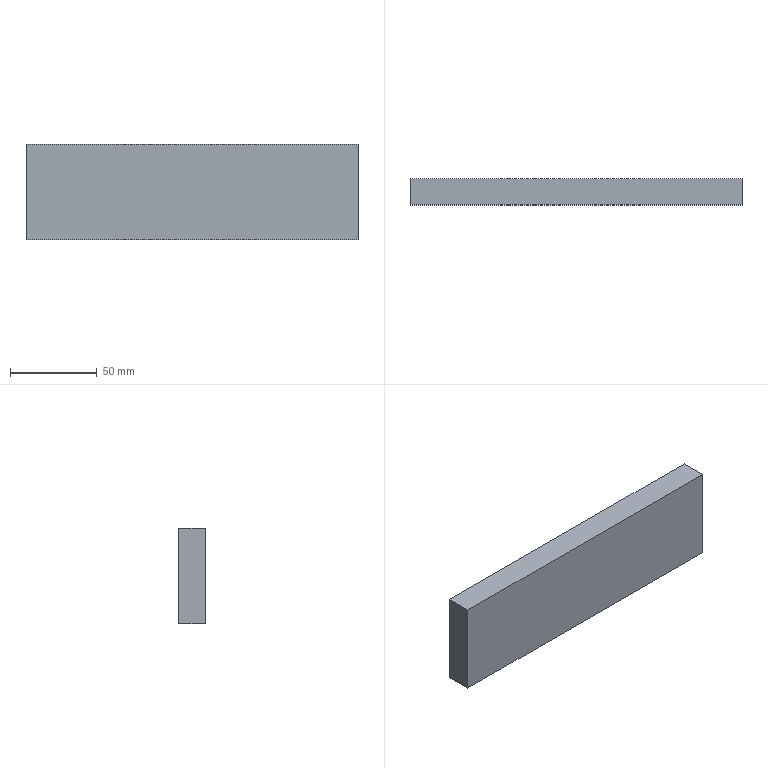Part | SolidWorks | features FlatPattern 1, SMBaseFlange 1, SheetMetal 1 | 1 solid | 6 faces | box 191 x 15 x 55 mm | volume 157575 mm3 | plane 6
STEP:
#1=CARTESIAN_POINT('',(0.,0.,0.));
#2=VERTEX_POINT('',#1);
#3=CARTESIAN_POINT('',(0.,0.,55.));
#4=VERTEX_POINT('',#3);
#5=CARTESIAN_POINT('',(0.,0.,0.));
#6=DIRECTION('',(0.,0.,1.));
#7=VECTOR('',#6,1000.);
#8=LINE('',#5,#7);
#9=EDGE_CURVE('',#2,#4,#8,.T.);
#10=ORIENTED_EDGE('',*,*,#9,.F.);
#11=CARTESIAN_POINT('',(0.,-15.,0.));
#12=VERTEX_POINT('',#11);
#13=CARTESIAN_POINT('',(0.,-15.,0.));
#14=DIRECTION('',(0.,1.,0.));
#15=VECTOR('',#14,1000.);
#16=LINE('',#13,#15);
#17=EDGE_CURVE('',#12,#2,#16,.T.);
#18=ORIENTED_EDGE('',*,*,#17,.F.);
#19=CARTESIAN_POINT('',(0.,-15.,55.));
#20=VERTEX_POINT('',#19);
#21=CARTESIAN_POINT('',(0.,-15.,0.));
#22=DIRECTION('',(0.,0.,1.));
#23=VECTOR('',#22,1000.);
#24=LINE('',#21,#23);
#25=EDGE_CURVE('',#12,#20,#24,.T.);
#26=ORIENTED_EDGE('',*,*,#25,.T.);
#27=CARTESIAN_POINT('',(0.,-15.,55.));
#28=DIRECTION('',(0.,1.,0.));
#29=VECTOR('',#28,1000.);
#30=LINE('',#27,#29);
#31=EDGE_CURVE('',#20,#4,#30,.T.);
#32=ORIENTED_EDGE('',*,*,#31,.T.);
#33=EDGE_LOOP('',(#10,#18,#26,#32));
#34=FACE_OUTER_BOUND('',#33,.T.);
#35=CARTESIAN_POINT('',(0.,-15.,0.));
#36=DIRECTION('',(-1.,0.,0.));
#37=DIRECTION('',(0.,0.,1.));
#38=AXIS2_PLACEMENT_3D('',#35,#36,#37);
#39=PLANE('',#38);
#40=ADVANCED_FACE('',(#34),#39,.T.);
#41=CARTESIAN_POINT('',(191.,0.,0.));
#42=VERTEX_POINT('',#41);
#43=CARTESIAN_POINT('',(0.,0.,0.));
#44=DIRECTION('',(-1.,0.,0.));
#45=VECTOR('',#44,1000.);
#46=LINE('',#43,#45);
#47=EDGE_CURVE('',#42,#2,#46,.T.);
#48=ORIENTED_EDGE('',*,*,#47,.F.);
#49=CARTESIAN_POINT('',(191.,-15.,0.));
#50=VERTEX_POINT('',#49);
#51=CARTESIAN_POINT('',(191.,-15.,0.));
#52=DIRECTION('',(0.,1.,0.));
#53=VECTOR('',#52,1000.);
#54=LINE('',#51,#53);
#55=EDGE_CURVE('',#50,#42,#54,.T.);
#56=ORIENTED_EDGE('',*,*,#55,.F.);
#57=CARTESIAN_POINT('',(0.,-15.,0.));
#58=DIRECTION('',(-1.,0.,0.));
#59=VECTOR('',#58,1000.);
#60=LINE('',#57,#59);
#61=EDGE_CURVE('',#50,#12,#60,.T.);
#62=ORIENTED_EDGE('',*,*,#61,.T.);
#63=ORIENTED_EDGE('',*,*,#17,.T.);
#64=EDGE_LOOP('',(#48,#56,#62,#63));
#65=FACE_OUTER_BOUND('',#64,.T.);
#66=CARTESIAN_POINT('',(0.,-15.,0.));
#67=DIRECTION('',(0.,0.,-1.));
#68=DIRECTION('',(-1.,0.,0.));
#69=AXIS2_PLACEMENT_3D('',#66,#67,#68);
#70=PLANE('',#69);
#71=ADVANCED_FACE('',(#65),#70,.T.);
#72=CARTESIAN_POINT('',(191.,0.,55.));
#73=VERTEX_POINT('',#72);
#74=CARTESIAN_POINT('',(191.,0.,0.));
#75=DIRECTION('',(0.,0.,-1.));
#76=VECTOR('',#75,1000.);
#77=LINE('',#74,#76);
#78=EDGE_CURVE('',#73,#42,#77,.T.);
#79=ORIENTED_EDGE('',*,*,#78,.F.);
#80=CARTESIAN_POINT('',(191.,-15.,55.));
#81=VERTEX_POINT('',#80);
#82=CARTESIAN_POINT('',(191.,-15.,55.));
#83=DIRECTION('',(0.,1.,0.));
#84=VECTOR('',#83,1000.);
#85=LINE('',#82,#84);
#86=EDGE_CURVE('',#81,#73,#85,.T.);
#87=ORIENTED_EDGE('',*,*,#86,.F.);
#88=CARTESIAN_POINT('',(191.,-15.,0.));
#89=DIRECTION('',(0.,0.,-1.));
#90=VECTOR('',#89,1000.);
#91=LINE('',#88,#90);
#92=EDGE_CURVE('',#81,#50,#91,.T.);
#93=ORIENTED_EDGE('',*,*,#92,.T.);
#94=ORIENTED_EDGE('',*,*,#55,.T.);
#95=EDGE_LOOP('',(#79,#87,#93,#94));
#96=FACE_OUTER_BOUND('',#95,.T.);
#97=CARTESIAN_POINT('',(191.,-15.,0.));
#98=DIRECTION('',(1.,0.,0.));
#99=DIRECTION('',(0.,0.,-1.));
#100=AXIS2_PLACEMENT_3D('',#97,#98,#99);
#101=PLANE('',#100);
#102=ADVANCED_FACE('',(#96),#101,.T.);
#103=CARTESIAN_POINT('',(0.,0.,55.));
#104=DIRECTION('',(1.,0.,0.));
#105=VECTOR('',#104,1000.);
#106=LINE('',#103,#105);
#107=EDGE_CURVE('',#4,#73,#106,.T.);
#108=ORIENTED_EDGE('',*,*,#107,.F.);
#109=ORIENTED_EDGE('',*,*,#31,.F.);
#110=CARTESIAN_POINT('',(0.,-15.,55.));
#111=DIRECTION('',(1.,0.,0.));
#112=VECTOR('',#111,1000.);
#113=LINE('',#110,#112);
#114=EDGE_CURVE('',#20,#81,#113,.T.);
#115=ORIENTED_EDGE('',*,*,#114,.T.);
#116=ORIENTED_EDGE('',*,*,#86,.T.);
#117=EDGE_LOOP('',(#108,#109,#115,#116));
#118=FACE_OUTER_BOUND('',#117,.T.);
#119=CARTESIAN_POINT('',(0.,-15.,55.));
#120=DIRECTION('',(0.,0.,1.));
#121=DIRECTION('',(1.,0.,0.));
#122=AXIS2_PLACEMENT_3D('',#119,#120,#121);
#123=PLANE('',#122);
#124=ADVANCED_FACE('',(#118),#123,.T.);
#125=ORIENTED_EDGE('',*,*,#25,.F.);
#126=ORIENTED_EDGE('',*,*,#61,.F.);
#127=ORIENTED_EDGE('',*,*,#92,.F.);
#128=ORIENTED_EDGE('',*,*,#114,.F.);
#129=EDGE_LOOP('',(#125,#126,#127,#128));
#130=FACE_OUTER_BOUND('',#129,.T.);
#131=CARTESIAN_POINT('',(0.,-15.,0.));
#132=DIRECTION('',(0.,1.,0.));
#133=DIRECTION('',(0.,0.,1.));
#134=AXIS2_PLACEMENT_3D('',#131,#132,#133);
#135=PLANE('',#134);
#136=ADVANCED_FACE('',(#130),#135,.F.);
#137=ORIENTED_EDGE('',*,*,#9,.T.);
#138=ORIENTED_EDGE('',*,*,#107,.T.);
#139=ORIENTED_EDGE('',*,*,#78,.T.);
#140=ORIENTED_EDGE('',*,*,#47,.T.);
#141=EDGE_LOOP('',(#137,#138,#139,#140));
#142=FACE_OUTER_BOUND('',#141,.T.);
#143=CARTESIAN_POINT('',(0.,0.,0.));
#144=DIRECTION('',(0.,1.,0.));
#145=DIRECTION('',(0.,0.,1.));
#146=AXIS2_PLACEMENT_3D('',#143,#144,#145);
#147=PLANE('',#146);
#148=ADVANCED_FACE('',(#142),#147,.T.);
#149=CLOSED_SHELL('',(#40,#71,#102,#124,#136,#148));
#150=MANIFOLD_SOLID_BREP('',#149);
#151=CARTESIAN_POINT('',(0.,0.,0.));
#152=DIRECTION('',(0.,0.,1.));
#153=DIRECTION('',(1.,0.,0.));
#154=AXIS2_PLACEMENT_3D('',#151,#152,#153);
#155=(LENGTH_UNIT()NAMED_UNIT(*)SI_UNIT(.MILLI.,.METRE.));
#156=UNCERTAINTY_MEASURE_WITH_UNIT(LENGTH_MEASURE(0.00001),#155,'','');
#157=(NAMED_UNIT(*)PLANE_ANGLE_UNIT()SI_UNIT($,.RADIAN.));
#158=(NAMED_UNIT(*)SI_UNIT($,.STERADIAN.)SOLID_ANGLE_UNIT());
#159=(GEOMETRIC_REPRESENTATION_CONTEXT(3)GLOBAL_UNCERTAINTY_ASSIGNED_CONTEXT((#156))GLOBAL_UNIT_ASSIGNED_CONTEXT((#155,#157,#158))REPRESENTATION_CONTEXT('',''));
#160=ADVANCED_BREP_SHAPE_REPRESENTATION('',(#150,#154),#159);